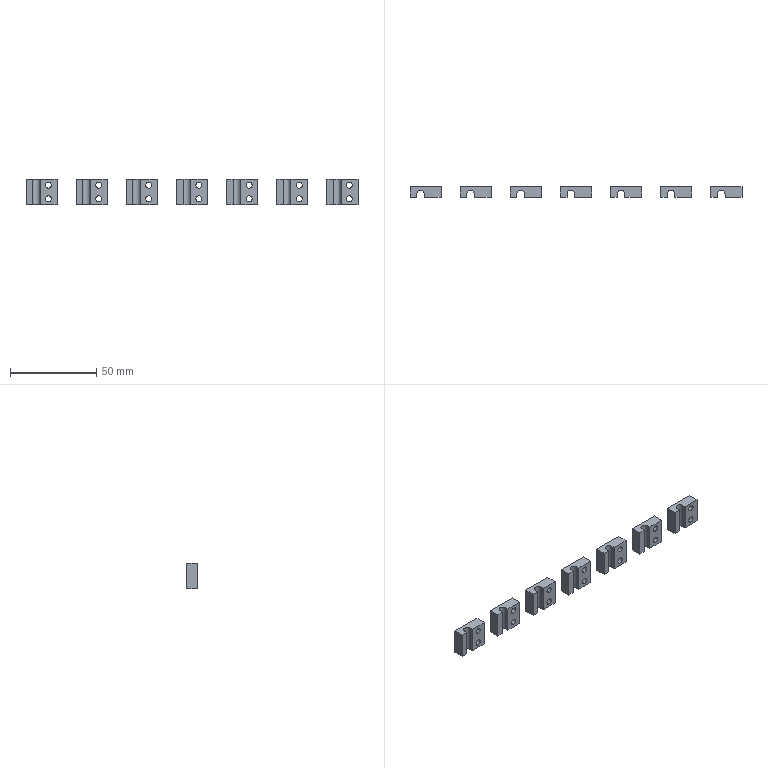NC program | Mastercam | posted with a generic post | part box 192 x 6 x 15 mm
Lines 6141 to 8014 of 12453:
(3 BM/BNOS |TOOL - 5|DIA. OFF. - 5|LEN. - 5|TOOL DIA. - 3.)
N2448 T5 M6
N2450 G0 G54 G90 X-61.688 Y9. C0. B0. S7000 M3
N2452 G43 H5 Z25.
N2454 Z1.569
N2456 G1 Z-3.431 F1000.
N2458 Y7.5 F3000.
N2460 Y-7.5
N2462 Y-9.
N2464 X-61.683
N2466 Z-3.455
N2468 Y-7.5
N2470 Y7.5
N2472 Y9.
N2474 X-61.677
N2476 Z-3.479
N2478 Y7.5
N2480 Y-7.5
N2482 Y-9.
N2484 X-61.67
N2486 Z-3.504
N2488 Y-7.5
N2490 Y7.5
N2492 Y9.
N2494 X-61.661
N2496 Z-3.527
N2498 Y7.5
N2500 Z-3.529
N2502 Y-7.5
N2504 Z-3.527
N2506 Y-9.
N2508 Z-3.529
N2510 X-61.652
N2512 Z-3.554
N2514 Y-7.5
N2516 Y7.5
N2518 Y9.
N2520 X-61.641
N2522 Z-3.579
N2524 Y7.5
N2526 Z-3.58
N2528 Y-7.5
N2530 Z-3.579
N2532 Y-9.
N2534 Z-3.58
N2536 X-61.63
N2538 Z-3.604
N2540 Y-7.5
N2542 Z-3.606
N2544 Y7.5
N2546 Z-3.604
N2548 Y9.
N2550 Z-3.606
N2552 X-61.616
N2554 Z-3.631
N2556 Y7.5
N2558 Z-3.632
N2560 Y-7.5
N2562 Z-3.631
N2564 Y-9.
N2566 Z-3.632
N2568 X-61.601
N2570 Z-3.656
N2572 Y-7.5
N2574 Z-3.658
N2576 Y7.5
N2578 Z-3.656
N2580 Y9.
N2582 Z-3.658
N2584 X-61.585
N2586 Z-3.681
N2588 Y7.5
N2590 Z-3.685
N2592 Y-7.5
N2594 Z-3.681
N2596 Y-9.
N2598 Z-3.685
N2600 X-61.567
N2602 Z-3.709
N2604 Y-7.5
N2606 Z-3.711
N2608 Y7.5
N2610 Z-3.709
N2612 Y9.
N2614 Z-3.711
N2616 X-61.55
N2618 Z-3.733
N2620 Y7.5
N2622 Y-7.5
N2624 Y-9.
N2626 X-61.534
N2628 Z-3.753
N2630 Y-7.5
N2632 Y7.5
N2634 Y9.
N2636 X-61.516
N2638 Z-3.773
N2640 Y7.5
N2642 Y-7.5
N2644 Y-9.
N2646 X-61.498
N2648 Z-3.792
N2650 Y-7.5
N2652 Y7.5
N2654 Y9.
N2656 X-61.479
N2658 Z-3.81
N2660 Y7.5
N2662 Z-3.811
N2664 Y-7.5
N2666 Z-3.81
N2668 Y-9.
N2670 Z-3.811
N2672 X-61.458
N2674 Z-3.829
N2676 Y-7.5
N2678 Y7.5
N2680 Y9.
N2682 X-61.437
N2684 Z-3.846
N2686 Y7.5
N2688 Z-3.847
N2690 Y-7.5
N2692 Z-3.846
N2694 Y-9.
N2696 Z-3.847
N2698 X-61.414
N2700 Z-3.864
N2702 Y-7.5
N2704 Y7.5
N2706 Y9.
N2708 X-61.391
N2710 Z-3.881
N2712 Y7.5
N2714 Y-7.5
N2716 Y-9.
N2718 X-61.366
N2720 Z-3.896
N2722 Y-7.5
N2724 Z-3.897
N2726 Y7.5
N2728 Z-3.896
N2730 Y9.
N2732 Z-3.897
N2734 X-61.341
N2736 Z-3.911
N2738 Y7.5
N2740 Z-3.912
N2742 Y-7.5
N2744 Z-3.911
N2746 Y-9.
N2748 Z-3.912
N2750 X-61.314
N2752 Z-3.925
N2754 Y-7.5
N2756 Y7.5
N2758 Y9.
N2760 X-61.287
N2762 Z-3.937
N2764 Y7.5
N2766 Z-3.938
N2768 Y-7.5
N2770 Z-3.937
N2772 Y-9.
N2774 Z-3.938
N2776 X-61.259
N2778 Z-3.95
N2780 Y-7.5
N2782 Y7.5
N2784 Y9.
N2786 X-61.231
N2788 Z-3.96
N2790 Y7.5
N2792 Z-3.961
N2794 Y-7.5
N2796 Z-3.96
N2798 Y-9.
N2800 Z-3.961
N2802 X-61.201
N2804 Z-3.969
N2806 Y-7.5
N2808 Z-3.97
N2810 Y7.5
N2812 Z-3.969
N2814 Y9.
N2816 Z-3.97
N2818 X-61.171
N2820 Z-3.979
N2822 Y7.5
N2824 Y-7.5
N2826 Y-9.
N2828 X-61.141
N2830 Z-3.984
N2832 Y-7.5
N2834 Z-3.986
N2836 Y7.5
N2838 Z-3.984
N2840 Y9.
N2842 Z-3.986
N2844 X-61.11
N2846 Z-3.99
N2848 Y7.5
N2850 Z-3.991
N2852 Y-7.5
N2854 Z-3.99
N2856 Y-9.
N2858 Z-3.991
N2860 X-61.079
N2862 Z-3.995
N2864 Y-7.5
N2866 Z-3.996
N2868 Y7.5
N2870 Z-3.995
N2872 Y9.
N2874 Z-3.996
N2876 X-61.047
N2878 Z-3.997
N2880 Y7.5
N2882 Z-3.998
N2884 Y-7.5
N2886 Z-3.997
N2888 Y-9.
N2890 Z-3.998
N2892 X-61.016
N2894 Z-3.999
N2896 Y-7.5
N2898 Z-4.
N2900 Y7.5
N2902 Z-3.999
N2904 Y9.
N2906 Z-4.
N2908 X-60.984
N2910 Z-3.999
N2912 Y7.5
N2914 Z-4.
N2916 Y-7.5
N2918 Z-3.999
N2920 Y-9.
N2922 Z-3.998
N2924 X-60.953
N2926 Z-3.997
N2928 Y-7.5
N2930 Z-3.998
N2932 Y7.5
N2934 Z-3.997
N2936 Y9.
N2938 Z-3.996
N2940 X-60.921
N2942 Z-3.995
N2944 Y7.5
N2946 Z-3.996
N2948 Y-7.5
N2950 Z-3.995
N2952 Y-9.
N2954 Z-3.991
N2956 X-60.89
N2958 Z-3.99
N2960 Y-7.5
N2962 Z-3.991
N2964 Y7.5
N2966 Z-3.99
N2968 Y9.
N2970 Z-3.986
N2972 X-60.859
N2974 Z-3.984
N2976 Y7.5
N2978 Z-3.986
N2980 Y-7.5
N2982 Z-3.984
N2984 Y-9.
N2986 Z-3.979
N2988 X-60.829
N2990 Y-7.5
N2992 Y7.5
N2994 Y9.
N2996 Z-3.97
N2998 X-60.799
N3000 Z-3.969
N3002 Y7.5
N3004 Z-3.97
N3006 Y-7.5
N3008 Z-3.969
N3010 Y-9.
N3012 Z-3.961
N3014 X-60.769
N3016 Z-3.96
N3018 Y-7.5
N3020 Z-3.961
N3022 Y7.5
N3024 Z-3.96
N3026 Y9.
N3028 Z-3.95
N3030 X-60.741
N3032 Y7.5
N3034 Y-7.5
N3036 Y-9.
N3038 Z-3.938
N3040 X-60.713
N3042 Z-3.937
N3044 Y-7.5
N3046 Z-3.938
N3048 Y7.5
N3050 Z-3.937
N3052 Y9.
N3054 Z-3.925
N3056 X-60.686
N3058 Y7.5
N3060 Y-7.5
N3062 Y-9.
N3064 Z-3.912
N3066 X-60.659
N3068 Z-3.911
N3070 Y-7.5
N3072 Z-3.912
N3074 Y7.5
N3076 Z-3.911
N3078 Y9.
N3080 Z-3.897
N3082 X-60.634
N3084 Z-3.896
N3086 Y7.5
N3088 Z-3.897
N3090 Y-7.5
N3092 Z-3.896
N3094 Y-9.
N3096 Z-3.881
N3098 X-60.609
N3100 Y-7.5
N3102 Y7.5
N3104 Y9.
N3106 Z-3.864
N3108 X-60.586
N3110 Y7.5
N3112 Y-7.5
N3114 Y-9.
N3116 Z-3.847
N3118 X-60.563
N3120 Z-3.846
N3122 Y-7.5
N3124 Z-3.847
N3126 Y7.5
N3128 Z-3.846
N3130 Y9.
N3132 Z-3.829
N3134 X-60.542
N3136 Y7.5
N3138 Y-7.5
N3140 Y-9.
N3142 Z-3.811
N3144 X-60.521
N3146 Z-3.81
N3148 Y-7.5
N3150 Z-3.811
N3152 Y7.5
N3154 Z-3.81
N3156 Y9.
N3158 Z-3.792
N3160 X-60.502
N3162 Y7.5
N3164 Y-7.5
N3166 Y-9.
N3168 Z-3.773
N3170 X-60.484
N3172 Y-7.5
N3174 Y7.5
N3176 Y9.
N3178 Z-3.753
N3180 X-60.466
N3182 Y7.5
N3184 Y-7.5
N3186 Y-9.
N3188 Z-3.733
N3190 X-60.45
N3192 Y-7.5
N3194 Y7.5
N3196 Y9.
N3198 Z-3.711
N3200 X-60.433
N3202 Z-3.709
N3204 Y7.5
N3206 Z-3.711
N3208 Y-7.5
N3210 Z-3.709
N3212 Y-9.
N3214 Z-3.685
N3216 X-60.415
N3218 Z-3.681
N3220 Y-7.5
N3222 Z-3.685
N3224 Y7.5
N3226 Z-3.681
N3228 Y9.
N3230 Z-3.658
N3232 X-60.399
N3234 Z-3.656
N3236 Y7.5
N3238 Z-3.658
N3240 Y-7.5
N3242 Z-3.656
N3244 Y-9.
N3246 Z-3.632
N3248 X-60.384
N3250 Z-3.631
N3252 Y-7.5
N3254 Z-3.632
N3256 Y7.5
N3258 Z-3.631
N3260 Y9.
N3262 Z-3.606
N3264 X-60.37
N3266 Z-3.604
N3268 Y7.5
N3270 Z-3.606
N3272 Y-7.5
N3274 Z-3.604
N3276 Y-9.
N3278 Z-3.58
N3280 X-60.359
N3282 Z-3.579
N3284 Y-7.5
N3286 Z-3.58
N3288 Y7.5
N3290 Z-3.579
N3292 Y9.
N3294 Z-3.554
N3296 X-60.348
N3298 Y7.5
N3300 Y-7.5
N3302 Y-9.
N3304 Z-3.529
N3306 X-60.339
N3308 Z-3.527
N3310 Y-7.5
N3312 Z-3.529
N3314 Y7.5
N3316 Z-3.527
N3318 Y9.
N3320 Z-3.504
N3322 X-60.33
N3324 Y7.5
N3326 Y-7.5
N3328 Y-9.
N3330 Z-3.479
N3332 X-60.323
N3334 Y-7.5
N3336 Y7.5
N3338 Y9.
N3340 Z-3.455
N3342 X-60.317
N3344 Y7.5
N3346 Y-7.5
N3348 Y-9.
N3350 Z-3.431
N3352 X-60.312
N3354 Y-7.5
N3356 Y7.5
N3358 Y9.
N3360 G0 Z1.569
N3362 Z25.
N3364 X-32.688
N3366 Z1.569
N3368 G1 Z-3.431 F1000.
N3370 Y7.5 F3000.
N3372 Y-7.5
N3374 Y-9.
N3376 X-32.683
N3378 Z-3.455
N3380 Y-7.5
N3382 Y7.5
N3384 Y9.
N3386 X-32.677
N3388 Z-3.479
N3390 Y7.5
N3392 Y-7.5
N3394 Y-9.
N3396 X-32.67
N3398 Z-3.504
N3400 Y-7.5
N3402 Y7.5
N3404 Y9.
N3406 X-32.661
N3408 Z-3.527
N3410 Y7.5
N3412 Z-3.529
N3414 Y-7.5
N3416 Z-3.527
N3418 Y-9.
N3420 Z-3.529
N3422 X-32.652
N3424 Z-3.554
N3426 Y-7.5
N3428 Y7.5
N3430 Y9.
N3432 X-32.641
N3434 Z-3.579
N3436 Y7.5
N3438 Z-3.58
N3440 Y-7.5
N3442 Z-3.579
N3444 Y-9.
N3446 Z-3.58
N3448 X-32.63
N3450 Z-3.604
N3452 Y-7.5
N3454 Z-3.606
N3456 Y7.5
N3458 Z-3.604
N3460 Y9.
N3462 Z-3.606
N3464 X-32.616
N3466 Z-3.631
N3468 Y7.5
N3470 Z-3.632
N3472 Y-7.5
N3474 Z-3.631
N3476 Y-9.
N3478 Z-3.632
N3480 X-32.601
N3482 Z-3.656
N3484 Y-7.5
N3486 Z-3.658
N3488 Y7.5
N3490 Z-3.656
N3492 Y9.
N3494 Z-3.658
N3496 X-32.585
N3498 Z-3.681
N3500 Y7.5
N3502 Z-3.685
N3504 Y-7.5
N3506 Z-3.681
N3508 Y-9.
N3510 Z-3.685
N3512 X-32.567
N3514 Z-3.709
N3516 Y-7.5
N3518 Z-3.711
N3520 Y7.5
N3522 Z-3.709
N3524 Y9.
N3526 Z-3.711
N3528 X-32.55
N3530 Z-3.733
N3532 Y7.5
N3534 Y-7.5
N3536 Y-9.
N3538 X-32.534
N3540 Z-3.753
N3542 Y-7.5
N3544 Y7.5
N3546 Y9.
N3548 X-32.516
N3550 Z-3.773
N3552 Y7.5
N3554 Y-7.5
N3556 Y-9.
N3558 X-32.498
N3560 Z-3.792
N3562 Y-7.5
N3564 Y7.5
N3566 Y9.
N3568 X-32.479
N3570 Z-3.81
N3572 Y7.5
N3574 Z-3.811
N3576 Y-7.5
N3578 Z-3.81
N3580 Y-9.
N3582 Z-3.811
N3584 X-32.458
N3586 Z-3.829
N3588 Y-7.5
N3590 Y7.5
N3592 Y9.
N3594 X-32.437
N3596 Z-3.846
N3598 Y7.5
N3600 Z-3.847
N3602 Y-7.5
N3604 Z-3.846
N3606 Y-9.
N3608 Z-3.847
N3610 X-32.414
N3612 Z-3.864
N3614 Y-7.5
N3616 Y7.5
N3618 Y9.
N3620 X-32.391
N3622 Z-3.881
N3624 Y7.5
N3626 Y-7.5
N3628 Y-9.
N3630 X-32.366
N3632 Z-3.896
N3634 Y-7.5
N3636 Z-3.897
N3638 Y7.5
N3640 Z-3.896
N3642 Y9.
N3644 Z-3.897
N3646 X-32.341
N3648 Z-3.911
N3650 Y7.5
N3652 Z-3.912
N3654 Y-7.5
N3656 Z-3.911
N3658 Y-9.
N3660 Z-3.912
N3662 X-32.314
N3664 Z-3.925
N3666 Y-7.5
N3668 Y7.5
N3670 Y9.
N3672 X-32.287
N3674 Z-3.937
N3676 Y7.5
N3678 Z-3.938
N3680 Y-7.5
N3682 Z-3.937
N3684 Y-9.
N3686 Z-3.938
N3688 X-32.259
N3690 Z-3.95
N3692 Y-7.5
N3694 Y7.5
N3696 Y9.
N3698 X-32.231
N3700 Z-3.96
N3702 Y7.5
N3704 Z-3.961
N3706 Y-7.5
N3708 Z-3.96
N3710 Y-9.
N3712 Z-3.961
N3714 X-32.201
N3716 Z-3.969
N3718 Y-7.5
N3720 Z-3.97
N3722 Y7.5
N3724 Z-3.969
N3726 Y9.
N3728 Z-3.97
N3730 X-32.171
N3732 Z-3.979
N3734 Y7.5
N3736 Y-7.5
N3738 Y-9.
N3740 X-32.141
N3742 Z-3.984
N3744 Y-7.5
N3746 Z-3.986
N3748 Y7.5
N3750 Z-3.984
N3752 Y9.
N3754 Z-3.986
N3756 X-32.11
N3758 Z-3.99
N3760 Y7.5
N3762 Z-3.991
N3764 Y-7.5
N3766 Z-3.99
N3768 Y-9.
N3770 Z-3.991
N3772 X-32.079
N3774 Z-3.995
N3776 Y-7.5
N3778 Z-3.996
N3780 Y7.5
N3782 Z-3.995
N3784 Y9.
N3786 Z-3.996
N3788 X-32.047
N3790 Z-3.997
N3792 Y7.5
N3794 Z-3.998
N3796 Y-7.5
N3798 Z-3.997
N3800 Y-9.
N3802 Z-3.998
N3804 X-32.016
N3806 Z-3.999
N3808 Y-7.5
N3810 Z-4.
N3812 Y7.5
N3814 Z-3.999
N3816 Y9.
N3818 Z-4.
N3820 X-31.984
N3822 Z-3.999
N3824 Y7.5
N3826 Z-4.
N3828 Y-7.5
N3830 Z-3.999
N3832 Y-9.
N3834 Z-3.998
N3836 X-31.953
N3838 Z-3.997
N3840 Y-7.5
N3842 Z-3.998
N3844 Y7.5
N3846 Z-3.997
N3848 Y9.
N3850 Z-3.996
N3852 X-31.921
N3854 Z-3.995
N3856 Y7.5
N3858 Z-3.996
N3860 Y-7.5
N3862 Z-3.995
N3864 Y-9.
N3866 Z-3.991
N3868 X-31.89
N3870 Z-3.99
N3872 Y-7.5
N3874 Z-3.991
N3876 Y7.5
N3878 Z-3.99
N3880 Y9.
N3882 Z-3.986
N3884 X-31.859
N3886 Z-3.984
N3888 Y7.5
N3890 Z-3.986
N3892 Y-7.5
N3894 Z-3.984
N3896 Y-9.
N3898 Z-3.979
N3900 X-31.829
N3902 Y-7.5
N3904 Y7.5
N3906 Y9.
N3908 Z-3.97
N3910 X-31.799
N3912 Z-3.969
N3914 Y7.5
N3916 Z-3.97
N3918 Y-7.5
N3920 Z-3.969
N3922 Y-9.
N3924 Z-3.961
N3926 X-31.769
N3928 Z-3.96
N3930 Y-7.5
N3932 Z-3.961
N3934 Y7.5
N3936 Z-3.96
N3938 Y9.
N3940 Z-3.95
N3942 X-31.741
N3944 Y7.5
N3946 Y-7.5
N3948 Y-9.
N3950 Z-3.938
N3952 X-31.713
N3954 Z-3.937
N3956 Y-7.5
N3958 Z-3.938
N3960 Y7.5
N3962 Z-3.937
N3964 Y9.
N3966 Z-3.925
N3968 X-31.686
N3970 Y7.5
N3972 Y-7.5
N3974 Y-9.
N3976 Z-3.912
N3978 X-31.659
N3980 Z-3.911
N3982 Y-7.5
N3984 Z-3.912
N3986 Y7.5
N3988 Z-3.911
N3990 Y9.
N3992 Z-3.897
N3994 X-31.634
N3996 Z-3.896
N3998 Y7.5
N4000 Z-3.897
N4002 Y-7.5
N4004 Z-3.896
N4006 Y-9.
N4008 Z-3.881
N4010 X-31.609
N4012 Y-7.5
N4014 Y7.5
N4016 Y9.
N4018 Z-3.864
N4020 X-31.586
N4022 Y7.5
N4024 Y-7.5
N4026 Y-9.
N4028 Z-3.847
N4030 X-31.563
N4032 Z-3.846
N4034 Y-7.5
N4036 Z-3.847
N4038 Y7.5
N4040 Z-3.846
N4042 Y9.
N4044 Z-3.829
N4046 X-31.542
N4048 Y7.5
N4050 Y-7.5
N4052 Y-9.
N4054 Z-3.811
N4056 X-31.521
N4058 Z-3.81
N4060 Y-7.5
N4062 Z-3.811
N4064 Y7.5
N4066 Z-3.81
N4068 Y9.
N4070 Z-3.792
N4072 X-31.502
N4074 Y7.5
N4076 Y-7.5
N4078 Y-9.
N4080 Z-3.773
N4082 X-31.484
N4084 Y-7.5
N4086 Y7.5
N4088 Y9.
N4090 Z-3.753
N4092 X-31.466
N4094 Y7.5
N4096 Y-7.5
N4098 Y-9.
N4100 Z-3.733
N4102 X-31.45
N4104 Y-7.5
N4106 Y7.5
N4108 Y9.
N4110 Z-3.711
N4112 X-31.433
N4114 Z-3.709
N4116 Y7.5
N4118 Z-3.711
N4120 Y-7.5
N4122 Z-3.709
N4124 Y-9.
N4126 Z-3.685
N4128 X-31.415
N4130 Z-3.681
N4132 Y-7.5
N4134 Z-3.685
N4136 Y7.5
N4138 Z-3.681
N4140 Y9.
N4142 Z-3.658
N4144 X-31.399
N4146 Z-3.656
N4148 Y7.5
N4150 Z-3.658
N4152 Y-7.5
N4154 Z-3.656
N4156 Y-9.
N4158 Z-3.632
N4160 X-31.384
N4162 Z-3.631
N4164 Y-7.5
N4166 Z-3.632
N4168 Y7.5
N4170 Z-3.631
N4172 Y9.
N4174 Z-3.606
N4176 X-31.37
N4178 Z-3.604
N4180 Y7.5
N4182 Z-3.606
N4184 Y-7.5
N4186 Z-3.604
N4188 Y-9.
N4190 Z-3.58
N4192 X-31.359
N4194 Z-3.579
N4196 Y-7.5
N4198 Z-3.58
N4200 Y7.5
N4202 Z-3.579
N4204 Y9.
N4206 Z-3.554
N4208 X-31.348
N4210 Y7.5
N4212 Y-7.5
N4214 Y-9.
N4216 Z-3.529
N4218 X-31.339
N4220 Z-3.527
N4222 Y-7.5
N4224 Z-3.529
N4226 Y7.5
N4228 Z-3.527
N4230 Y9.
N4232 Z-3.504
N4234 X-31.33
N4236 Y7.5
N4238 Y-7.5
N4240 Y-9.
N4242 Z-3.479
N4244 X-31.323
N4246 Y-7.5
N4248 Y7.5
N4250 Y9.
N4252 Z-3.455
N4254 X-31.317
N4256 Y7.5
N4258 Y-7.5
N4260 Y-9.
N4262 Z-3.431
N4264 X-31.312
N4266 Y-7.5
N4268 Y7.5
N4270 Y9.
N4272 G0 Z1.569
N4274 Z25.
N4276 X-3.688
N4278 Z1.569
N4280 G1 Z-3.431 F1000.
N4282 Y7.5 F3000.
N4284 Y-7.5
N4286 Y-9.
N4288 X-3.683
N4290 Z-3.455
N4292 Y-7.5
N4294 Y7.5
N4296 Y9.
N4298 X-3.677
N4300 Z-3.479
N4302 Y7.5
N4304 Y-7.5
N4306 Y-9.
N4308 X-3.67
N4310 Z-3.504
N4312 Y-7.5
N4314 Y7.5
N4316 Y9.
N4318 X-3.661
N4320 Z-3.527
N4322 Y7.5
N4324 Z-3.529
N4326 Y-7.5
N4328 Z-3.527
N4330 Y-9.
N4332 Z-3.529
N4334 X-3.652
N4336 Z-3.554
N4338 Y-7.5
N4340 Y7.5
N4342 Y9.
N4344 X-3.641
N4346 Z-3.579
N4348 Y7.5
N4350 Z-3.58
N4352 Y-7.5
N4354 Z-3.579
N4356 Y-9.
N4358 Z-3.58
N4360 X-3.63
N4362 Z-3.604
N4364 Y-7.5
N4366 Z-3.606
N4368 Y7.5
N4370 Z-3.604
N4372 Y9.
N4374 Z-3.606
N4376 X-3.616
N4378 Z-3.631
N4380 Y7.5
N4382 Z-3.632
N4384 Y-7.5
N4386 Z-3.631
N4388 Y-9.
N4390 Z-3.632
N4392 X-3.601
N4394 Z-3.656
N4396 Y-7.5
N4398 Z-3.658
N4400 Y7.5
N4402 Z-3.656
N4404 Y9.
N4406 Z-3.658
N4408 X-3.585
N4410 Z-3.681
N4412 Y7.5
N4414 Z-3.685
N4416 Y-7.5
N4418 Z-3.681
N4420 Y-9.
N4422 Z-3.685
N4424 X-3.567
N4426 Z-3.709
N4428 Y-7.5
N4430 Z-3.711
N4432 Y7.5
N4434 Z-3.709
N4436 Y9.
N4438 Z-3.711
N4440 X-3.55
N4442 Z-3.733
N4444 Y7.5
N4446 Y-7.5
N4448 Y-9.
N4450 X-3.534
N4452 Z-3.753
N4454 Y-7.5
N4456 Y7.5
N4458 Y9.
N4460 X-3.516
N4462 Z-3.773
N4464 Y7.5
N4466 Y-7.5
N4468 Y-9.
N4470 X-3.498
N4472 Z-3.792
N4474 Y-7.5
N4476 Y7.5
N4478 Y9.
N4480 X-3.479
N4482 Z-3.81
N4484 Y7.5
N4486 Z-3.811
N4488 Y-7.5
N4490 Z-3.81
N4492 Y-9.
N4494 Z-3.811
N4496 X-3.458
N4498 Z-3.829
N4500 Y-7.5
N4502 Y7.5
N4504 Y9.
N4506 X-3.437
N4508 Z-3.846
N4510 Y7.5
N4512 Z-3.847
N4514 Y-7.5
N4516 Z-3.846
N4518 Y-9.
N4520 Z-3.847
N4522 X-3.414
N4524 Z-3.864
N4526 Y-7.5
N4528 Y7.5
N4530 Y9.
N4532 X-3.391
N4534 Z-3.881
N4536 Y7.5
N4538 Y-7.5
N4540 Y-9.
N4542 X-3.366
N4544 Z-3.896
N4546 Y-7.5
N4548 Z-3.897
N4550 Y7.5
N4552 Z-3.896
N4554 Y9.
N4556 Z-3.897
N4558 X-3.341
N4560 Z-3.911
N4562 Y7.5
N4564 Z-3.912
N4566 Y-7.5
N4568 Z-3.911
N4570 Y-9.
N4572 Z-3.912
N4574 X-3.314
N4576 Z-3.925
N4578 Y-7.5
N4580 Y7.5
N4582 Y9.
N4584 X-3.287
N4586 Z-3.937
N4588 Y7.5
N4590 Z-3.938
N4592 Y-7.5
N4594 Z-3.937
N4596 Y-9.
N4598 Z-3.938
N4600 X-3.259
N4602 Z-3.95
N4604 Y-7.5
N4606 Y7.5
N4608 Y9.
N4610 X-3.231
N4612 Z-3.96
N4614 Y7.5
N4616 Z-3.961
N4618 Y-7.5
N4620 Z-3.96
N4622 Y-9.
N4624 Z-3.961
N4626 X-3.201
N4628 Z-3.969
N4630 Y-7.5
N4632 Z-3.97
N4634 Y7.5
N4636 Z-3.969
N4638 Y9.
N4640 Z-3.97
N4642 X-3.171
N4644 Z-3.979
N4646 Y7.5
N4648 Y-7.5
N4650 Y-9.
N4652 X-3.141
N4654 Z-3.984
N4656 Y-7.5
N4658 Z-3.986
N4660 Y7.5
N4662 Z-3.984
N4664 Y9.
N4666 Z-3.986
N4668 X-3.11
N4670 Z-3.99
N4672 Y7.5
N4674 Z-3.991
N4676 Y-7.5
N4678 Z-3.99
N4680 Y-9.
N4682 Z-3.991
N4684 X-3.079
N4686 Z-3.995
N4688 Y-7.5
N4690 Z-3.996
N4692 Y7.5
N4694 Z-3.995
N4696 Y9.
N4698 Z-3.996
N4700 X-3.047
N4702 Z-3.997
N4704 Y7.5
N4706 Z-3.998
N4708 Y-7.5
N4710 Z-3.997
N4712 Y-9.
N4714 Z-3.998
N4716 X-3.016
N4718 Z-3.999
N4720 Y-7.5
N4722 Z-4.
N4724 Y7.5
N4726 Z-3.999
N4728 Y9.
N4730 Z-4.
N4732 X-2.984
N4734 Z-3.999
N4736 Y7.5
N4738 Z-4.
N4740 Y-7.5
N4742 Z-3.999
N4744 Y-9.
N4746 Z-3.998
N4748 X-2.953
N4750 Z-3.997
N4752 Y-7.5
N4754 Z-3.998
N4756 Y7.5
N4758 Z-3.997
N4760 Y9.
N4762 Z-3.996
N4764 X-2.921
N4766 Z-3.995
N4768 Y7.5
N4770 Z-3.996
N4772 Y-7.5
N4774 Z-3.995
N4776 Y-9.
N4778 Z-3.991
N4780 X-2.89
N4782 Z-3.99
N4784 Y-7.5
N4786 Z-3.991
N4788 Y7.5
N4790 Z-3.99
N4792 Y9.
N4794 Z-3.986
N4796 X-2.859
N4798 Z-3.984
N4800 Y7.5
N4802 Z-3.986
N4804 Y-7.5
N4806 Z-3.984
N4808 Y-9.
N4810 Z-3.979
N4812 X-2.829
N4814 Y-7.5
N4816 Y7.5
N4818 Y9.
N4820 Z-3.97
N4822 X-2.799
N4824 Z-3.969
N4826 Y7.5
N4828 Z-3.97
N4830 Y-7.5
N4832 Z-3.969
N4834 Y-9.
N4836 Z-3.961
N4838 X-2.769
N4840 Z-3.96
N4842 Y-7.5
N4844 Z-3.961
N4846 Y7.5
N4848 Z-3.96
N4850 Y9.
N4852 Z-3.95
N4854 X-2.741
N4856 Y7.5
N4858 Y-7.5
N4860 Y-9.
N4862 Z-3.938
N4864 X-2.713
N4866 Z-3.937
N4868 Y-7.5
N4870 Z-3.938
N4872 Y7.5
N4874 Z-3.937
N4876 Y9.
N4878 Z-3.925
N4880 X-2.686
N4882 Y7.5
N4884 Y-7.5
N4886 Y-9.
N4888 Z-3.912
N4890 X-2.659
N4892 Z-3.911
N4894 Y-7.5
N4896 Z-3.912
N4898 Y7.5
N4900 Z-3.911
N4902 Y9.
N4904 Z-3.897
N4906 X-2.634
N4908 Z-3.896
N4910 Y7.5
N4912 Z-3.897
N4914 Y-7.5
N4916 Z-3.896
N4918 Y-9.
N4920 Z-3.881
N4922 X-2.609
N4924 Y-7.5
N4926 Y7.5
N4928 Y9.
N4930 Z-3.864
N4932 X-2.586
N4934 Y7.5
N4936 Y-7.5
N4938 Y-9.
N4940 Z-3.847
N4942 X-2.563
N4944 Z-3.846
N4946 Y-7.5
N4948 Z-3.847
N4950 Y7.5
N4952 Z-3.846
N4954 Y9.
N4956 Z-3.829
N4958 X-2.542
N4960 Y7.5
N4962 Y-7.5
N4964 Y-9.
N4966 Z-3.811
N4968 X-2.521
N4970 Z-3.81
N4972 Y-7.5
N4974 Z-3.811
N4976 Y7.5
N4978 Z-3.81
N4980 Y9.
N4982 Z-3.792
N4984 X-2.502
N4986 Y7.5
N4988 Y-7.5
N4990 Y-9.
N4992 Z-3.773
N4994 X-2.484
N4996 Y-7.5
N4998 Y7.5
N5000 Y9.
N5002 Z-3.753
N5004 X-2.466
N5006 Y7.5
N5008 Y-7.5
N5010 Y-9.
N5012 Z-3.733
N5014 X-2.45
N5016 Y-7.5
N5018 Y7.5
N5020 Y9.
N5022 Z-3.711
N5024 X-2.433
N5026 Z-3.709
N5028 Y7.5
N5030 Z-3.711
N5032 Y-7.5
N5034 Z-3.709
N5036 Y-9.
N5038 Z-3.685
N5040 X-2.415
N5042 Z-3.681
N5044 Y-7.5
N5046 Z-3.685
N5048 Y7.5
N5050 Z-3.681
N5052 Y9.
N5054 Z-3.658
N5056 X-2.399
N5058 Z-3.656
N5060 Y7.5
N5062 Z-3.658
N5064 Y-7.5
N5066 Z-3.656
N5068 Y-9.
N5070 Z-3.632
N5072 X-2.384
N5074 Z-3.631
N5076 Y-7.5
N5078 Z-3.632
N5080 Y7.5
N5082 Z-3.631
N5084 Y9.
N5086 Z-3.606
N5088 X-2.37
N5090 Z-3.604
N5092 Y7.5
N5094 Z-3.606
N5096 Y-7.5
N5098 Z-3.604
N5100 Y-9.
N5102 Z-3.58
N5104 X-2.359
N5106 Z-3.579
N5108 Y-7.5
N5110 Z-3.58
N5112 Y7.5
N5114 Z-3.579
N5116 Y9.
N5118 Z-3.554
N5120 X-2.348
N5122 Y7.5
N5124 Y-7.5
N5126 Y-9.
N5128 Z-3.529
N5130 X-2.339
N5132 Z-3.527
N5134 Y-7.5
N5136 Z-3.529
N5138 Y7.5
N5140 Z-3.527
N5142 Y9.
N5144 Z-3.504
N5146 X-2.33
N5148 Y7.5
N5150 Y-7.5
N5152 Y-9.
N5154 Z-3.479
N5156 X-2.323
N5158 Y-7.5
N5160 Y7.5
N5162 Y9.
N5164 Z-3.455
N5166 X-2.317
N5168 Y7.5
N5170 Y-7.5
N5172 Y-9.
N5174 Z-3.431
N5176 X-2.312
N5178 Y-7.5
N5180 Y7.5
N5182 Y9.
N5184 G0 Z1.569
N5186 Z25.
N5188 X25.312
N5190 Z1.569
N5192 G1 Z-3.431 F1000.
N5194 Y7.5 F3000.
N5196 Y-7.5
N5198 Y-9.
N5200 X25.317
N5202 Z-3.455
N5204 Y-7.5
N5206 Y7.5
N5208 Y9.
N5210 X25.323
N5212 Z-3.479
N5214 Y7.5
N5216 Y-7.5
N5218 Y-9.
N5220 X25.33
N5222 Z-3.504
N5224 Y-7.5
N5226 Y7.5
N5228 Y9.
N5230 X25.339
N5232 Z-3.527
N5234 Y7.5
N5236 Z-3.529
N5238 Y-7.5
N5240 Z-3.527
N5242 Y-9.
N5244 Z-3.529
N5246 X25.348
N5248 Z-3.554
N5250 Y-7.5
N5252 Y7.5
N5254 Y9.
N5256 X25.359
N5258 Z-3.579
N5260 Y7.5
N5262 Z-3.58
N5264 Y-7.5
N5266 Z-3.579
N5268 Y-9.
N5270 Z-3.58
N5272 X25.37
N5274 Z-3.604
N5276 Y-7.5
N5278 Z-3.606
N5280 Y7.5
N5282 Z-3.604
N5284 Y9.
N5286 Z-3.606
N5288 X25.384
N5290 Z-3.631
N5292 Y7.5
N5294 Z-3.632
N5296 Y-7.5
N5298 Z-3.631
N5300 Y-9.
N5302 Z-3.632
N5304 X25.399
N5306 Z-3.656
N5308 Y-7.5
N5310 Z-3.658
N5312 Y7.5
N5314 Z-3.656
N5316 Y9.
N5318 Z-3.658
N5320 X25.415
N5322 Z-3.681
N5324 Y7.5
N5326 Z-3.685
N5328 Y-7.5
N5330 Z-3.681
N5332 Y-9.
N5334 Z-3.685
N5336 X25.433
N5338 Z-3.709
N5340 Y-7.5
N5342 Z-3.711
N5344 Y7.5
N5346 Z-3.709
N5348 Y9.
N5350 Z-3.711
N5352 X25.45
N5354 Z-3.733
N5356 Y7.5
N5358 Y-7.5
N5360 Y-9.
N5362 X25.466
N5364 Z-3.753
N5366 Y-7.5
N5368 Y7.5
N5370 Y9.
N5372 X25.484
N5374 Z-3.773
N5376 Y7.5
N5378 Y-7.5
N5380 Y-9.
N5382 X25.502
N5384 Z-3.792
N5386 Y-7.5
N5388 Y7.5
N5390 Y9.
N5392 X25.521
N5394 Z-3.81
N5396 Y7.5
N5398 Z-3.811
N5400 Y-7.5
N5402 Z-3.81
N5404 Y-9.
N5406 Z-3.811
N5408 X25.542
N5410 Z-3.829
N5412 Y-7.5
N5414 Y7.5
N5416 Y9.
N5418 X25.563
N5420 Z-3.846
N5422 Y7.5
N5424 Z-3.847
N5426 Y-7.5
N5428 Z-3.846
N5430 Y-9.
N5432 Z-3.847
N5434 X25.586
N5436 Z-3.864
N5438 Y-7.5
N5440 Y7.5
N5442 Y9.
N5444 X25.609
N5446 Z-3.881
N5448 Y7.5
N5450 Y-7.5
N5452 Y-9.
N5454 X25.634
N5456 Z-3.896
N5458 Y-7.5
N5460 Z-3.897
N5462 Y7.5
N5464 Z-3.896
N5466 Y9.
N5468 Z-3.897
N5470 X25.659
N5472 Z-3.911
N5474 Y7.5
N5476 Z-3.912
N5478 Y-7.5
N5480 Z-3.911
N5482 Y-9.
N5484 Z-3.912
N5486 X25.686
N5488 Z-3.925
N5490 Y-7.5
N5492 Y7.5
N5494 Y9.
N5496 X25.713
N5498 Z-3.937
N5500 Y7.5
N5502 Z-3.938
N5504 Y-7.5
N5506 Z-3.937
N5508 Y-9.
N5510 Z-3.938
N5512 X25.741
N5514 Z-3.95
N5516 Y-7.5
N5518 Y7.5
N5520 Y9.
N5522 X25.769
N5524 Z-3.96
N5526 Y7.5
N5528 Z-3.961
N5530 Y-7.5
N5532 Z-3.96
N5534 Y-9.
N5536 Z-3.961
N5538 X25.799
N5540 Z-3.969
N5542 Y-7.5
N5544 Z-3.97
N5546 Y7.5
N5548 Z-3.969
N5550 Y9.
N5552 Z-3.97
N5554 X25.829
N5556 Z-3.979
N5558 Y7.5
N5560 Y-7.5
N5562 Y-9.
N5564 X25.859
N5566 Z-3.984
N5568 Y-7.5
N5570 Z-3.986
N5572 Y7.5
N5574 Z-3.984
N5576 Y9.
N5578 Z-3.986
N5580 X25.89
N5582 Z-3.99
N5584 Y7.5
N5586 Z-3.991
N5588 Y-7.5
N5590 Z-3.99
N5592 Y-9.
N5594 Z-3.991
N5596 X25.921
N5598 Z-3.995
N5600 Y-7.5
N5602 Z-3.996
N5604 Y7.5
N5606 Z-3.995
N5608 Y9.
N5610 Z-3.996
N5612 X25.953
N5614 Z-3.997
N5616 Y7.5
N5618 Z-3.998
N5620 Y-7.5
N5622 Z-3.997
N5624 Y-9.
N5626 Z-3.998
N5628 X25.984
N5630 Z-3.999
N5632 Y-7.5
N5634 Z-4.
N5636 Y7.5
N5638 Z-3.999
N5640 Y9.
N5642 Z-4.
N5644 X26.016
N5646 Z-3.999
N5648 Y7.5
N5650 Z-4.
N5652 Y-7.5
N5654 Z-3.999
N5656 Y-9.
N5658 Z-3.998
N5660 X26.047
N5662 Z-3.997
N5664 Y-7.5
N5666 Z-3.998
N5668 Y7.5
N5670 Z-3.997
N5672 Y9.
N5674 Z-3.996
N5676 X26.079
N5678 Z-3.995
N5680 Y7.5
N5682 Z-3.996
N5684 Y-7.5
N5686 Z-3.995
N5688 Y-9.
N5690 Z-3.991
N5692 X26.11
N5694 Z-3.99
N5696 Y-7.5
N5698 Z-3.991
N5700 Y7.5
N5702 Z-3.99
N5704 Y9.
N5706 Z-3.986
N5708 X26.141
N5710 Z-3.984
N5712 Y7.5
N5714 Z-3.986
N5716 Y-7.5
N5718 Z-3.984
N5720 Y-9.
N5722 Z-3.979
N5724 X26.171
N5726 Y-7.5
N5728 Y7.5
N5730 Y9.
N5732 Z-3.97
N5734 X26.201
N5736 Z-3.969
N5738 Y7.5
N5740 Z-3.97
N5742 Y-7.5
N5744 Z-3.969
N5746 Y-9.
N5748 Z-3.961
N5750 X26.231
N5752 Z-3.96
N5754 Y-7.5
N5756 Z-3.961
N5758 Y7.5
N5760 Z-3.96
N5762 Y9.
N5764 Z-3.95
N5766 X26.259
N5768 Y7.5
N5770 Y-7.5
N5772 Y-9.
N5774 Z-3.938
N5776 X26.287
N5778 Z-3.937
N5780 Y-7.5
N5782 Z-3.938
N5784 Y7.5
N5786 Z-3.937
N5788 Y9.
N5790 Z-3.925
N5792 X26.314
N5794 Y7.5
N5796 Y-7.5
N5798 Y-9.
N5800 Z-3.912
N5802 X26.341
N5804 Z-3.911
N5806 Y-7.5
N5808 Z-3.912
N5810 Y7.5
N5812 Z-3.911
N5814 Y9.
N5816 Z-3.897
N5818 X26.366
N5820 Z-3.896
N5822 Y7.5
N5824 Z-3.897
N5826 Y-7.5
N5828 Z-3.896
N5830 Y-9.
N5832 Z-3.881
N5834 X26.391
N5836 Y-7.5
N5838 Y7.5
N5840 Y9.
N5842 Z-3.864
N5844 X26.414
N5846 Y7.5
N5848 Y-7.5
N5850 Y-9.
N5852 Z-3.847
N5854 X26.437
N5856 Z-3.846
N5858 Y-7.5
N5860 Z-3.847
N5862 Y7.5
N5864 Z-3.846
N5866 Y9.
N5868 Z-3.829
N5870 X26.458
N5872 Y7.5
N5874 Y-7.5
N5876 Y-9.
N5878 Z-3.811
N5880 X26.479
N5882 Z-3.81
N5884 Y-7.5
N5886 Z-3.811
N5888 Y7.5
N5890 Z-3.81
N5892 Y9.
N5894 Z-3.792
N5896 X26.498
N5898 Y7.5
N5900 Y-7.5
N5902 Y-9.
N5904 Z-3.773
N5906 X26.516
N5908 Y-7.5
N5910 Y7.5
N5912 Y9.
N5914 Z-3.753
N5916 X26.534
N5918 Y7.5
N5920 Y-7.5
N5922 Y-9.
N5924 Z-3.733
N5926 X26.55
N5928 Y-7.5
N5930 Y7.5
N5932 Y9.
N5934 Z-3.711
N5936 X26.567
N5938 Z-3.709
N5940 Y7.5
N5942 Z-3.711
N5944 Y-7.5
N5946 Z-3.709
N5948 Y-9.
N5950 Z-3.685
N5952 X26.585
N5954 Z-3.681
N5956 Y-7.5
N5958 Z-3.685
N5960 Y7.5
N5962 Z-3.681
N5964 Y9.
N5966 Z-3.658
N5968 X26.601
N5970 Z-3.656
N5972 Y7.5
N5974 Z-3.658
N5976 Y-7.5
N5978 Z-3.656
N5980 Y-9.
N5982 Z-3.632
N5984 X26.616
N5986 Z-3.631
N5988 Y-7.5
N5990 Z-3.632
N5992 Y7.5
N5994 Z-3.631
N5996 Y9.
N5998 Z-3.606
N6000 X26.63
N6002 Z-3.604
N6004 Y7.5
N6006 Z-3.606
N6008 Y-7.5
N6010 Z-3.604
N6012 Y-9.
N6014 Z-3.58
N6016 X26.641
N6018 Z-3.579
N6020 Y-7.5
N6022 Z-3.58
N6024 Y7.5
N6026 Z-3.579
N6028 Y9.
N6030 Z-3.554
N6032 X26.652
N6034 Y7.5
N6036 Y-7.5
N6038 Y-9.
N6040 Z-3.529
N6042 X26.661
N6044 Z-3.527
N6046 Y-7.5
N6048 Z-3.529
N6050 Y7.5
N6052 Z-3.527
N6054 Y9.
N6056 Z-3.504
N6058 X26.67
N6060 Y7.5
N6062 Y-7.5
N6064 Y-9.
N6066 Z-3.479
N6068 X26.677
N6070 Y-7.5
N6072 Y7.5
N6074 Y9.
N6076 Z-3.455
N6078 X26.683
N6080 Y7.5
N6082 Y-7.5
N6084 Y-9.
N6086 Z-3.431
N6088 X26.688
N6090 Y-7.5
N6092 Y7.5
N6094 Y9.
N6096 G0 Z1.569
N6098 Z25.
N6100 X54.312
N6102 Z1.569
N6104 G1 Z-3.431 F1000.
N6106 Y7.5 F3000.
N6108 Y-7.5
N6110 Y-9.
N6112 X54.317
N6114 Z-3.455
N6116 Y-7.5
N6118 Y7.5
N6120 Y9.
N6122 X54.323
N6124 Z-3.479
N6126 Y7.5
N6128 Y-7.5
N6130 Y-9.
N6132 X54.33
N6134 Z-3.504
N6136 Y-7.5
N6138 Y7.5
N6140 Y9.
N6142 X54.339
N6144 Z-3.527
N6146 Y7.5
N6148 Z-3.529
N6150 Y-7.5
N6152 Z-3.527
N6154 Y-9.
N6156 Z-3.529
N6158 X54.348
N6160 Z-3.554
N6162 Y-7.5
N6164 Y7.5
N6166 Y9.
N6168 X54.359
N6170 Z-3.579
N6172 Y7.5
N6174 Z-3.58
N6176 Y-7.5
N6178 Z-3.579
N6180 Y-9.
N6182 Z-3.58
N6184 X54.37
N6186 Z-3.604
N6188 Y-7.5
N6190 Z-3.606
N6192 Y7.5